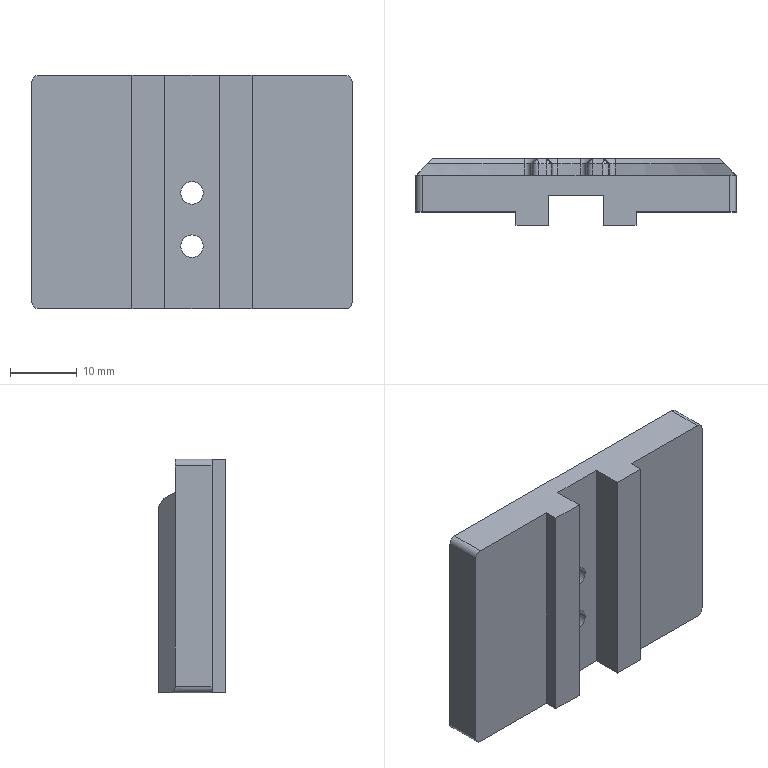Part | STEP file | product positioning block B | 1 solid | 65 faces | box 48 x 10 x 35 mm | volume 11917 mm3 | plane 27 | cylinder 25 | cone 13 | commonest cylinder face diameters 1.6 x8 2 x4 3.4 x4 6 x4 96 x3 89 x2